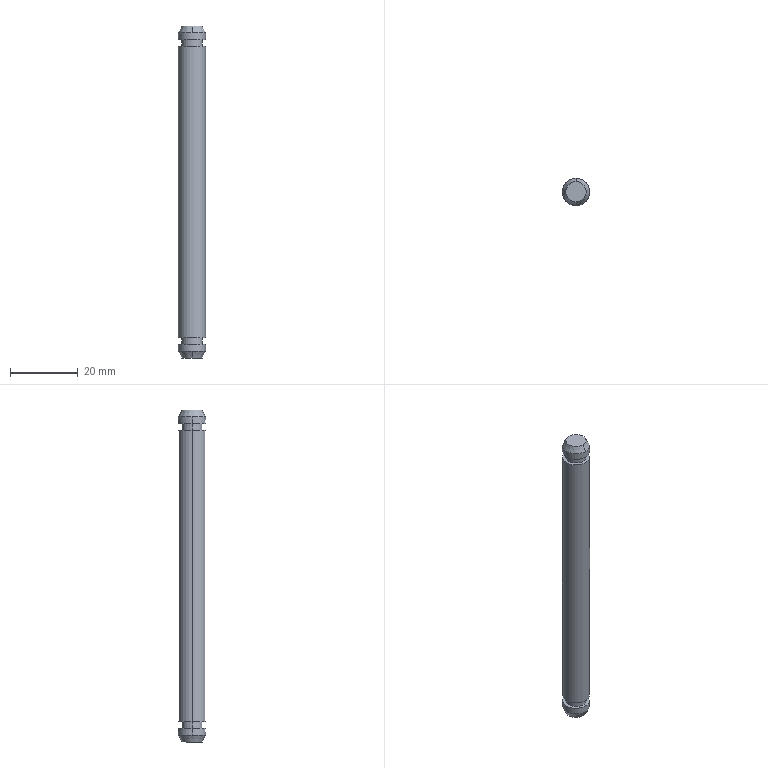Part | SolidWorks | features BaseBody 1 | 1 solid | 20 faces | box 8 x 8 x 98 mm | volume 4792 mm3 | cylinder 10 | plane 6 | cone 4 | commonest cylinder face diameters 8 x6 6 x4
STEP:
#1=CARTESIAN_POINT('',(4.,0.,-43.));
#2=VERTEX_POINT('',#1);
#3=CARTESIAN_POINT('',(-4.,0.,-43.));
#4=VERTEX_POINT('',#3);
#5=CARTESIAN_POINT('',(0.,0.,-43.));
#6=DIRECTION('',(0.,0.,1.));
#7=DIRECTION('',(1.,0.,0.));
#8=AXIS2_PLACEMENT_3D('',#5,#6,#7);
#9=CIRCLE('',#8,4.);
#10=EDGE_CURVE('',#2,#4,#9,.T.);
#11=ORIENTED_EDGE('',*,*,#10,.T.);
#12=CARTESIAN_POINT('',(-4.,0.,43.));
#13=VERTEX_POINT('',#12);
#14=CARTESIAN_POINT('',(-4.,0.,0.));
#15=DIRECTION('',(0.,0.,1.));
#16=VECTOR('',#15,1000.);
#17=LINE('',#14,#16);
#18=EDGE_CURVE('',#4,#13,#17,.T.);
#19=ORIENTED_EDGE('',*,*,#18,.T.);
#20=CARTESIAN_POINT('',(4.,0.,43.));
#21=VERTEX_POINT('',#20);
#22=CARTESIAN_POINT('',(0.,0.,43.));
#23=DIRECTION('',(0.,0.,-1.));
#24=DIRECTION('',(1.,0.,0.));
#25=AXIS2_PLACEMENT_3D('',#22,#23,#24);
#26=CIRCLE('',#25,4.);
#27=EDGE_CURVE('',#13,#21,#26,.T.);
#28=ORIENTED_EDGE('',*,*,#27,.T.);
#29=CARTESIAN_POINT('',(4.,0.,0.));
#30=DIRECTION('',(0.,0.,1.));
#31=VECTOR('',#30,1000.);
#32=LINE('',#29,#31);
#33=EDGE_CURVE('',#2,#21,#32,.T.);
#34=ORIENTED_EDGE('',*,*,#33,.F.);
#35=EDGE_LOOP('',(#11,#19,#28,#34));
#36=FACE_OUTER_BOUND('',#35,.T.);
#37=CARTESIAN_POINT('',(0.,0.,0.));
#38=DIRECTION('',(0.,0.,1.));
#39=DIRECTION('',(1.,0.,0.));
#40=AXIS2_PLACEMENT_3D('',#37,#38,#39);
#41=CYLINDRICAL_SURFACE('',#40,4.);
#42=ADVANCED_FACE('',(#36),#41,.T.);
#43=CARTESIAN_POINT('',(-3.,0.,45.));
#44=VERTEX_POINT('',#43);
#45=CARTESIAN_POINT('',(3.,0.,45.));
#46=VERTEX_POINT('',#45);
#47=CARTESIAN_POINT('',(0.,0.,45.));
#48=DIRECTION('',(0.,0.,-1.));
#49=DIRECTION('',(-1.,0.,0.));
#50=AXIS2_PLACEMENT_3D('',#47,#48,#49);
#51=CIRCLE('',#50,3.);
#52=EDGE_CURVE('',#44,#46,#51,.T.);
#53=ORIENTED_EDGE('',*,*,#52,.T.);
#54=CARTESIAN_POINT('',(3.,0.,43.));
#55=VERTEX_POINT('',#54);
#56=CARTESIAN_POINT('',(3.,0.,0.));
#57=DIRECTION('',(0.,0.,-1.));
#58=VECTOR('',#57,1000.);
#59=LINE('',#56,#58);
#60=EDGE_CURVE('',#46,#55,#59,.T.);
#61=ORIENTED_EDGE('',*,*,#60,.T.);
#62=CARTESIAN_POINT('',(-3.,0.,43.));
#63=VERTEX_POINT('',#62);
#64=CARTESIAN_POINT('',(0.,0.,43.));
#65=DIRECTION('',(0.,0.,1.));
#66=DIRECTION('',(-1.,0.,0.));
#67=AXIS2_PLACEMENT_3D('',#64,#65,#66);
#68=CIRCLE('',#67,3.);
#69=EDGE_CURVE('',#55,#63,#68,.T.);
#70=ORIENTED_EDGE('',*,*,#69,.T.);
#71=CARTESIAN_POINT('',(-3.,0.,0.));
#72=DIRECTION('',(0.,0.,-1.));
#73=VECTOR('',#72,1000.);
#74=LINE('',#71,#73);
#75=EDGE_CURVE('',#44,#63,#74,.T.);
#76=ORIENTED_EDGE('',*,*,#75,.F.);
#77=EDGE_LOOP('',(#53,#61,#70,#76));
#78=FACE_OUTER_BOUND('',#77,.T.);
#79=CARTESIAN_POINT('',(0.,0.,0.));
#80=DIRECTION('',(0.,0.,-1.));
#81=DIRECTION('',(-1.,0.,0.));
#82=AXIS2_PLACEMENT_3D('',#79,#80,#81);
#83=CYLINDRICAL_SURFACE('',#82,3.);
#84=ADVANCED_FACE('',(#78),#83,.T.);
#85=CARTESIAN_POINT('',(3.,0.,-45.));
#86=VERTEX_POINT('',#85);
#87=CARTESIAN_POINT('',(-3.,0.,-45.));
#88=VERTEX_POINT('',#87);
#89=CARTESIAN_POINT('',(0.,0.,-45.));
#90=DIRECTION('',(0.,0.,1.));
#91=DIRECTION('',(1.,0.,0.));
#92=AXIS2_PLACEMENT_3D('',#89,#90,#91);
#93=CIRCLE('',#92,3.);
#94=EDGE_CURVE('',#86,#88,#93,.T.);
#95=ORIENTED_EDGE('',*,*,#94,.T.);
#96=CARTESIAN_POINT('',(-3.,0.,-43.));
#97=VERTEX_POINT('',#96);
#98=CARTESIAN_POINT('',(-3.,0.,0.));
#99=DIRECTION('',(0.,0.,1.));
#100=VECTOR('',#99,1000.);
#101=LINE('',#98,#100);
#102=EDGE_CURVE('',#88,#97,#101,.T.);
#103=ORIENTED_EDGE('',*,*,#102,.T.);
#104=CARTESIAN_POINT('',(3.,0.,-43.));
#105=VERTEX_POINT('',#104);
#106=CARTESIAN_POINT('',(0.,0.,-43.));
#107=DIRECTION('',(0.,0.,-1.));
#108=DIRECTION('',(1.,0.,0.));
#109=AXIS2_PLACEMENT_3D('',#106,#107,#108);
#110=CIRCLE('',#109,3.);
#111=EDGE_CURVE('',#97,#105,#110,.T.);
#112=ORIENTED_EDGE('',*,*,#111,.T.);
#113=CARTESIAN_POINT('',(3.,0.,0.));
#114=DIRECTION('',(0.,0.,1.));
#115=VECTOR('',#114,1000.);
#116=LINE('',#113,#115);
#117=EDGE_CURVE('',#86,#105,#116,.T.);
#118=ORIENTED_EDGE('',*,*,#117,.F.);
#119=EDGE_LOOP('',(#95,#103,#112,#118));
#120=FACE_OUTER_BOUND('',#119,.T.);
#121=CARTESIAN_POINT('',(0.,0.,0.));
#122=DIRECTION('',(0.,0.,1.));
#123=DIRECTION('',(1.,0.,0.));
#124=AXIS2_PLACEMENT_3D('',#121,#122,#123);
#125=CYLINDRICAL_SURFACE('',#124,3.);
#126=ADVANCED_FACE('',(#120),#125,.T.);
#127=CARTESIAN_POINT('',(0.,4.,47.));
#128=VERTEX_POINT('',#127);
#129=CARTESIAN_POINT('',(4.,0.,47.));
#130=VERTEX_POINT('',#129);
#131=CARTESIAN_POINT('',(0.,0.,47.));
#132=DIRECTION('',(0.,0.,-1.));
#133=DIRECTION('',(-1.,0.,0.));
#134=AXIS2_PLACEMENT_3D('',#131,#132,#133);
#135=CIRCLE('',#134,4.);
#136=EDGE_CURVE('',#128,#130,#135,.T.);
#137=ORIENTED_EDGE('',*,*,#136,.T.);
#138=CARTESIAN_POINT('',(4.,0.,45.));
#139=VERTEX_POINT('',#138);
#140=CARTESIAN_POINT('',(4.,0.,0.));
#141=DIRECTION('',(0.,0.,-1.));
#142=VECTOR('',#141,1000.);
#143=LINE('',#140,#142);
#144=EDGE_CURVE('',#130,#139,#143,.T.);
#145=ORIENTED_EDGE('',*,*,#144,.T.);
#146=CARTESIAN_POINT('',(-4.,0.,45.));
#147=VERTEX_POINT('',#146);
#148=CARTESIAN_POINT('',(0.,0.,45.));
#149=DIRECTION('',(0.,0.,1.));
#150=DIRECTION('',(-1.,0.,0.));
#151=AXIS2_PLACEMENT_3D('',#148,#149,#150);
#152=CIRCLE('',#151,4.);
#153=EDGE_CURVE('',#139,#147,#152,.T.);
#154=ORIENTED_EDGE('',*,*,#153,.T.);
#155=CARTESIAN_POINT('',(-4.,0.,47.));
#156=VERTEX_POINT('',#155);
#157=CARTESIAN_POINT('',(-4.,0.,0.));
#158=DIRECTION('',(0.,0.,-1.));
#159=VECTOR('',#158,1000.);
#160=LINE('',#157,#159);
#161=EDGE_CURVE('',#156,#147,#160,.T.);
#162=ORIENTED_EDGE('',*,*,#161,.F.);
#163=CARTESIAN_POINT('',(0.,0.,47.));
#164=DIRECTION('',(0.,0.,-1.));
#165=DIRECTION('',(-1.,0.,0.));
#166=AXIS2_PLACEMENT_3D('',#163,#164,#165);
#167=CIRCLE('',#166,4.);
#168=EDGE_CURVE('',#156,#128,#167,.T.);
#169=ORIENTED_EDGE('',*,*,#168,.T.);
#170=EDGE_LOOP('',(#137,#145,#154,#162,#169));
#171=FACE_OUTER_BOUND('',#170,.T.);
#172=CARTESIAN_POINT('',(0.,0.,0.));
#173=DIRECTION('',(0.,0.,-1.));
#174=DIRECTION('',(-1.,0.,0.));
#175=AXIS2_PLACEMENT_3D('',#172,#173,#174);
#176=CYLINDRICAL_SURFACE('',#175,4.);
#177=ADVANCED_FACE('',(#171),#176,.T.);
#178=CARTESIAN_POINT('',(0.,4.,-47.));
#179=VERTEX_POINT('',#178);
#180=CARTESIAN_POINT('',(-4.,0.,-47.));
#181=VERTEX_POINT('',#180);
#182=CARTESIAN_POINT('',(0.,0.,-47.));
#183=DIRECTION('',(0.,0.,1.));
#184=DIRECTION('',(1.,0.,0.));
#185=AXIS2_PLACEMENT_3D('',#182,#183,#184);
#186=CIRCLE('',#185,4.);
#187=EDGE_CURVE('',#179,#181,#186,.T.);
#188=ORIENTED_EDGE('',*,*,#187,.T.);
#189=CARTESIAN_POINT('',(-4.,0.,-45.));
#190=VERTEX_POINT('',#189);
#191=CARTESIAN_POINT('',(-4.,0.,0.));
#192=DIRECTION('',(0.,0.,1.));
#193=VECTOR('',#192,1000.);
#194=LINE('',#191,#193);
#195=EDGE_CURVE('',#181,#190,#194,.T.);
#196=ORIENTED_EDGE('',*,*,#195,.T.);
#197=CARTESIAN_POINT('',(4.,0.,-45.));
#198=VERTEX_POINT('',#197);
#199=CARTESIAN_POINT('',(0.,0.,-45.));
#200=DIRECTION('',(0.,0.,-1.));
#201=DIRECTION('',(1.,0.,0.));
#202=AXIS2_PLACEMENT_3D('',#199,#200,#201);
#203=CIRCLE('',#202,4.);
#204=EDGE_CURVE('',#190,#198,#203,.T.);
#205=ORIENTED_EDGE('',*,*,#204,.T.);
#206=CARTESIAN_POINT('',(4.,0.,-47.));
#207=VERTEX_POINT('',#206);
#208=CARTESIAN_POINT('',(4.,0.,0.));
#209=DIRECTION('',(0.,0.,1.));
#210=VECTOR('',#209,1000.);
#211=LINE('',#208,#210);
#212=EDGE_CURVE('',#207,#198,#211,.T.);
#213=ORIENTED_EDGE('',*,*,#212,.F.);
#214=CARTESIAN_POINT('',(0.,0.,-47.));
#215=DIRECTION('',(0.,0.,1.));
#216=DIRECTION('',(1.,0.,0.));
#217=AXIS2_PLACEMENT_3D('',#214,#215,#216);
#218=CIRCLE('',#217,4.);
#219=EDGE_CURVE('',#207,#179,#218,.T.);
#220=ORIENTED_EDGE('',*,*,#219,.T.);
#221=EDGE_LOOP('',(#188,#196,#205,#213,#220));
#222=FACE_OUTER_BOUND('',#221,.T.);
#223=CARTESIAN_POINT('',(0.,0.,0.));
#224=DIRECTION('',(0.,0.,1.));
#225=DIRECTION('',(1.,0.,0.));
#226=AXIS2_PLACEMENT_3D('',#223,#224,#225);
#227=CYLINDRICAL_SURFACE('',#226,4.);
#228=ADVANCED_FACE('',(#222),#227,.T.);
#229=CARTESIAN_POINT('',(0.,3.,49.));
#230=VERTEX_POINT('',#229);
#231=CARTESIAN_POINT('',(0.,-3.,49.));
#232=VERTEX_POINT('',#231);
#233=CARTESIAN_POINT('',(0.,0.,49.));
#234=DIRECTION('',(0.,0.,-1.));
#235=DIRECTION('',(0.,1.,0.));
#236=AXIS2_PLACEMENT_3D('',#233,#234,#235);
#237=CIRCLE('',#236,3.);
#238=EDGE_CURVE('',#230,#232,#237,.T.);
#239=ORIENTED_EDGE('',*,*,#238,.T.);
#240=CARTESIAN_POINT('',(0.,-4.,47.));
#241=VERTEX_POINT('',#240);
#242=CARTESIAN_POINT('',(0.,-4.,47.));
#243=DIRECTION('',(0.,-0.4472,-0.8944));
#244=VECTOR('',#243,1000.);
#245=LINE('',#242,#244);
#246=EDGE_CURVE('',#232,#241,#245,.T.);
#247=ORIENTED_EDGE('',*,*,#246,.T.);
#248=CARTESIAN_POINT('',(0.,0.,47.));
#249=DIRECTION('',(0.,0.,-1.));
#250=DIRECTION('',(-1.,0.,0.));
#251=AXIS2_PLACEMENT_3D('',#248,#249,#250);
#252=CIRCLE('',#251,4.);
#253=EDGE_CURVE('',#130,#241,#252,.T.);
#254=ORIENTED_EDGE('',*,*,#253,.F.);
#255=ORIENTED_EDGE('',*,*,#136,.F.);
#256=CARTESIAN_POINT('',(0.,4.,47.));
#257=DIRECTION('',(0.,0.4472,-0.8944));
#258=VECTOR('',#257,1000.);
#259=LINE('',#256,#258);
#260=EDGE_CURVE('',#230,#128,#259,.T.);
#261=ORIENTED_EDGE('',*,*,#260,.F.);
#262=EDGE_LOOP('',(#239,#247,#254,#255,#261));
#263=FACE_OUTER_BOUND('',#262,.T.);
#264=CARTESIAN_POINT('',(0.,0.,47.));
#265=DIRECTION('',(0.,0.,-1.));
#266=DIRECTION('',(0.,1.,0.));
#267=AXIS2_PLACEMENT_3D('',#264,#265,#266);
#268=CONICAL_SURFACE('',#267,4.,0.4636);
#269=ADVANCED_FACE('',(#263),#268,.T.);
#270=CARTESIAN_POINT('',(0.,-3.,-49.));
#271=VERTEX_POINT('',#270);
#272=CARTESIAN_POINT('',(0.,3.,-49.));
#273=VERTEX_POINT('',#272);
#274=CARTESIAN_POINT('',(0.,0.,-49.));
#275=DIRECTION('',(0.,0.,1.));
#276=DIRECTION('',(0.,-1.,0.));
#277=AXIS2_PLACEMENT_3D('',#274,#275,#276);
#278=CIRCLE('',#277,3.);
#279=EDGE_CURVE('',#271,#273,#278,.T.);
#280=ORIENTED_EDGE('',*,*,#279,.T.);
#281=CARTESIAN_POINT('',(0.,4.,-47.));
#282=DIRECTION('',(0.,0.4472,0.8944));
#283=VECTOR('',#282,1000.);
#284=LINE('',#281,#283);
#285=EDGE_CURVE('',#273,#179,#284,.T.);
#286=ORIENTED_EDGE('',*,*,#285,.T.);
#287=ORIENTED_EDGE('',*,*,#219,.F.);
#288=CARTESIAN_POINT('',(0.,-4.,-47.));
#289=VERTEX_POINT('',#288);
#290=CARTESIAN_POINT('',(0.,0.,-47.));
#291=DIRECTION('',(0.,0.,1.));
#292=DIRECTION('',(1.,0.,0.));
#293=AXIS2_PLACEMENT_3D('',#290,#291,#292);
#294=CIRCLE('',#293,4.);
#295=EDGE_CURVE('',#289,#207,#294,.T.);
#296=ORIENTED_EDGE('',*,*,#295,.F.);
#297=CARTESIAN_POINT('',(0.,-4.,-47.));
#298=DIRECTION('',(0.,-0.4472,0.8944));
#299=VECTOR('',#298,1000.);
#300=LINE('',#297,#299);
#301=EDGE_CURVE('',#271,#289,#300,.T.);
#302=ORIENTED_EDGE('',*,*,#301,.F.);
#303=EDGE_LOOP('',(#280,#286,#287,#296,#302));
#304=FACE_OUTER_BOUND('',#303,.T.);
#305=CARTESIAN_POINT('',(0.,0.,-47.));
#306=DIRECTION('',(0.,0.,1.));
#307=DIRECTION('',(0.,-1.,0.));
#308=AXIS2_PLACEMENT_3D('',#305,#306,#307);
#309=CONICAL_SURFACE('',#308,4.,0.4636);
#310=ADVANCED_FACE('',(#304),#309,.T.);
#311=ORIENTED_EDGE('',*,*,#18,.F.);
#312=CARTESIAN_POINT('',(0.,0.,-43.));
#313=DIRECTION('',(0.,0.,1.));
#314=DIRECTION('',(1.,0.,0.));
#315=AXIS2_PLACEMENT_3D('',#312,#313,#314);
#316=CIRCLE('',#315,4.);
#317=EDGE_CURVE('',#4,#2,#316,.T.);
#318=ORIENTED_EDGE('',*,*,#317,.T.);
#319=ORIENTED_EDGE('',*,*,#33,.T.);
#320=CARTESIAN_POINT('',(0.,0.,43.));
#321=DIRECTION('',(0.,0.,-1.));
#322=DIRECTION('',(1.,0.,0.));
#323=AXIS2_PLACEMENT_3D('',#320,#321,#322);
#324=CIRCLE('',#323,4.);
#325=EDGE_CURVE('',#21,#13,#324,.T.);
#326=ORIENTED_EDGE('',*,*,#325,.T.);
#327=EDGE_LOOP('',(#311,#318,#319,#326));
#328=FACE_OUTER_BOUND('',#327,.T.);
#329=CARTESIAN_POINT('',(0.,0.,0.));
#330=DIRECTION('',(0.,0.,1.));
#331=DIRECTION('',(1.,0.,0.));
#332=AXIS2_PLACEMENT_3D('',#329,#330,#331);
#333=CYLINDRICAL_SURFACE('',#332,4.);
#334=ADVANCED_FACE('',(#328),#333,.T.);
#335=ORIENTED_EDGE('',*,*,#325,.F.);
#336=ORIENTED_EDGE('',*,*,#27,.F.);
#337=EDGE_LOOP('',(#335,#336));
#338=FACE_OUTER_BOUND('',#337,.T.);
#339=CARTESIAN_POINT('',(0.,0.,43.));
#340=DIRECTION('',(0.,0.,1.));
#341=DIRECTION('',(-1.,0.,0.));
#342=AXIS2_PLACEMENT_3D('',#339,#340,#341);
#343=CIRCLE('',#342,3.);
#344=EDGE_CURVE('',#63,#55,#343,.T.);
#345=ORIENTED_EDGE('',*,*,#344,.F.);
#346=ORIENTED_EDGE('',*,*,#69,.F.);
#347=EDGE_LOOP('',(#345,#346));
#348=FACE_BOUND('',#347,.T.);
#349=CARTESIAN_POINT('',(0.,4.,43.));
#350=DIRECTION('',(0.,0.,-1.));
#351=DIRECTION('',(-1.,0.,0.));
#352=AXIS2_PLACEMENT_3D('',#349,#350,#351);
#353=PLANE('',#352);
#354=ADVANCED_FACE('',(#338,#348),#353,.F.);
#355=ORIENTED_EDGE('',*,*,#10,.F.);
#356=ORIENTED_EDGE('',*,*,#317,.F.);
#357=EDGE_LOOP('',(#355,#356));
#358=FACE_OUTER_BOUND('',#357,.T.);
#359=CARTESIAN_POINT('',(0.,0.,-43.));
#360=DIRECTION('',(0.,0.,-1.));
#361=DIRECTION('',(1.,0.,0.));
#362=AXIS2_PLACEMENT_3D('',#359,#360,#361);
#363=CIRCLE('',#362,3.);
#364=EDGE_CURVE('',#105,#97,#363,.T.);
#365=ORIENTED_EDGE('',*,*,#364,.F.);
#366=ORIENTED_EDGE('',*,*,#111,.F.);
#367=EDGE_LOOP('',(#365,#366));
#368=FACE_BOUND('',#367,.T.);
#369=CARTESIAN_POINT('',(0.,4.,-43.));
#370=DIRECTION('',(0.,0.,1.));
#371=DIRECTION('',(1.,0.,0.));
#372=AXIS2_PLACEMENT_3D('',#369,#370,#371);
#373=PLANE('',#372);
#374=ADVANCED_FACE('',(#358,#368),#373,.F.);
#375=ORIENTED_EDGE('',*,*,#60,.F.);
#376=CARTESIAN_POINT('',(0.,0.,45.));
#377=DIRECTION('',(0.,0.,-1.));
#378=DIRECTION('',(-1.,0.,0.));
#379=AXIS2_PLACEMENT_3D('',#376,#377,#378);
#380=CIRCLE('',#379,3.);
#381=EDGE_CURVE('',#46,#44,#380,.T.);
#382=ORIENTED_EDGE('',*,*,#381,.T.);
#383=ORIENTED_EDGE('',*,*,#75,.T.);
#384=ORIENTED_EDGE('',*,*,#344,.T.);
#385=EDGE_LOOP('',(#375,#382,#383,#384));
#386=FACE_OUTER_BOUND('',#385,.T.);
#387=CARTESIAN_POINT('',(0.,0.,0.));
#388=DIRECTION('',(0.,0.,-1.));
#389=DIRECTION('',(-1.,0.,0.));
#390=AXIS2_PLACEMENT_3D('',#387,#388,#389);
#391=CYLINDRICAL_SURFACE('',#390,3.);
#392=ADVANCED_FACE('',(#386),#391,.T.);
#393=ORIENTED_EDGE('',*,*,#102,.F.);
#394=CARTESIAN_POINT('',(0.,0.,-45.));
#395=DIRECTION('',(0.,0.,1.));
#396=DIRECTION('',(1.,0.,0.));
#397=AXIS2_PLACEMENT_3D('',#394,#395,#396);
#398=CIRCLE('',#397,3.);
#399=EDGE_CURVE('',#88,#86,#398,.T.);
#400=ORIENTED_EDGE('',*,*,#399,.T.);
#401=ORIENTED_EDGE('',*,*,#117,.T.);
#402=ORIENTED_EDGE('',*,*,#364,.T.);
#403=EDGE_LOOP('',(#393,#400,#401,#402));
#404=FACE_OUTER_BOUND('',#403,.T.);
#405=CARTESIAN_POINT('',(0.,0.,0.));
#406=DIRECTION('',(0.,0.,1.));
#407=DIRECTION('',(1.,0.,0.));
#408=AXIS2_PLACEMENT_3D('',#405,#406,#407);
#409=CYLINDRICAL_SURFACE('',#408,3.);
#410=ADVANCED_FACE('',(#404),#409,.T.);
#411=ORIENTED_EDGE('',*,*,#52,.F.);
#412=ORIENTED_EDGE('',*,*,#381,.F.);
#413=EDGE_LOOP('',(#411,#412));
#414=FACE_BOUND('',#413,.T.);
#415=CARTESIAN_POINT('',(0.,0.,45.));
#416=DIRECTION('',(0.,0.,1.));
#417=DIRECTION('',(-1.,0.,0.));
#418=AXIS2_PLACEMENT_3D('',#415,#416,#417);
#419=CIRCLE('',#418,4.);
#420=EDGE_CURVE('',#147,#139,#419,.T.);
#421=ORIENTED_EDGE('',*,*,#420,.F.);
#422=ORIENTED_EDGE('',*,*,#153,.F.);
#423=EDGE_LOOP('',(#421,#422));
#424=FACE_OUTER_BOUND('',#423,.T.);
#425=CARTESIAN_POINT('',(0.,3.,45.));
#426=DIRECTION('',(0.,0.,1.));
#427=DIRECTION('',(1.,0.,0.));
#428=AXIS2_PLACEMENT_3D('',#425,#426,#427);
#429=PLANE('',#428);
#430=ADVANCED_FACE('',(#414,#424),#429,.F.);
#431=ORIENTED_EDGE('',*,*,#94,.F.);
#432=ORIENTED_EDGE('',*,*,#399,.F.);
#433=EDGE_LOOP('',(#431,#432));
#434=FACE_BOUND('',#433,.T.);
#435=CARTESIAN_POINT('',(0.,0.,-45.));
#436=DIRECTION('',(0.,0.,-1.));
#437=DIRECTION('',(1.,0.,0.));
#438=AXIS2_PLACEMENT_3D('',#435,#436,#437);
#439=CIRCLE('',#438,4.);
#440=EDGE_CURVE('',#198,#190,#439,.T.);
#441=ORIENTED_EDGE('',*,*,#440,.F.);
#442=ORIENTED_EDGE('',*,*,#204,.F.);
#443=EDGE_LOOP('',(#441,#442));
#444=FACE_OUTER_BOUND('',#443,.T.);
#445=CARTESIAN_POINT('',(0.,3.,-45.));
#446=DIRECTION('',(0.,0.,-1.));
#447=DIRECTION('',(-1.,0.,0.));
#448=AXIS2_PLACEMENT_3D('',#445,#446,#447);
#449=PLANE('',#448);
#450=ADVANCED_FACE('',(#434,#444),#449,.F.);
#451=ORIENTED_EDGE('',*,*,#144,.F.);
#452=ORIENTED_EDGE('',*,*,#253,.T.);
#453=CARTESIAN_POINT('',(0.,0.,47.));
#454=DIRECTION('',(0.,0.,-1.));
#455=DIRECTION('',(-1.,0.,0.));
#456=AXIS2_PLACEMENT_3D('',#453,#454,#455);
#457=CIRCLE('',#456,4.);
#458=EDGE_CURVE('',#241,#156,#457,.T.);
#459=ORIENTED_EDGE('',*,*,#458,.T.);
#460=ORIENTED_EDGE('',*,*,#161,.T.);
#461=ORIENTED_EDGE('',*,*,#420,.T.);
#462=EDGE_LOOP('',(#451,#452,#459,#460,#461));
#463=FACE_OUTER_BOUND('',#462,.T.);
#464=CARTESIAN_POINT('',(0.,0.,0.));
#465=DIRECTION('',(0.,0.,-1.));
#466=DIRECTION('',(-1.,0.,0.));
#467=AXIS2_PLACEMENT_3D('',#464,#465,#466);
#468=CYLINDRICAL_SURFACE('',#467,4.);
#469=ADVANCED_FACE('',(#463),#468,.T.);
#470=ORIENTED_EDGE('',*,*,#195,.F.);
#471=CARTESIAN_POINT('',(0.,0.,-47.));
#472=DIRECTION('',(0.,0.,1.));
#473=DIRECTION('',(1.,0.,0.));
#474=AXIS2_PLACEMENT_3D('',#471,#472,#473);
#475=CIRCLE('',#474,4.);
#476=EDGE_CURVE('',#181,#289,#475,.T.);
#477=ORIENTED_EDGE('',*,*,#476,.T.);
#478=ORIENTED_EDGE('',*,*,#295,.T.);
#479=ORIENTED_EDGE('',*,*,#212,.T.);
#480=ORIENTED_EDGE('',*,*,#440,.T.);
#481=EDGE_LOOP('',(#470,#477,#478,#479,#480));
#482=FACE_OUTER_BOUND('',#481,.T.);
#483=CARTESIAN_POINT('',(0.,0.,0.));
#484=DIRECTION('',(0.,0.,1.));
#485=DIRECTION('',(1.,0.,0.));
#486=AXIS2_PLACEMENT_3D('',#483,#484,#485);
#487=CYLINDRICAL_SURFACE('',#486,4.);
#488=ADVANCED_FACE('',(#482),#487,.T.);
#489=ORIENTED_EDGE('',*,*,#246,.F.);
#490=CARTESIAN_POINT('',(0.,0.,49.));
#491=DIRECTION('',(0.,0.,-1.));
#492=DIRECTION('',(0.,1.,0.));
#493=AXIS2_PLACEMENT_3D('',#490,#491,#492);
#494=CIRCLE('',#493,3.);
#495=EDGE_CURVE('',#232,#230,#494,.T.);
#496=ORIENTED_EDGE('',*,*,#495,.T.);
#497=ORIENTED_EDGE('',*,*,#260,.T.);
#498=ORIENTED_EDGE('',*,*,#168,.F.);
#499=ORIENTED_EDGE('',*,*,#458,.F.);
#500=EDGE_LOOP('',(#489,#496,#497,#498,#499));
#501=FACE_OUTER_BOUND('',#500,.T.);
#502=CARTESIAN_POINT('',(0.,0.,47.));
#503=DIRECTION('',(0.,0.,-1.));
#504=DIRECTION('',(0.,1.,0.));
#505=AXIS2_PLACEMENT_3D('',#502,#503,#504);
#506=CONICAL_SURFACE('',#505,4.,0.4636);
#507=ADVANCED_FACE('',(#501),#506,.T.);
#508=ORIENTED_EDGE('',*,*,#285,.F.);
#509=CARTESIAN_POINT('',(0.,0.,-49.));
#510=DIRECTION('',(0.,0.,1.));
#511=DIRECTION('',(0.,-1.,0.));
#512=AXIS2_PLACEMENT_3D('',#509,#510,#511);
#513=CIRCLE('',#512,3.);
#514=EDGE_CURVE('',#273,#271,#513,.T.);
#515=ORIENTED_EDGE('',*,*,#514,.T.);
#516=ORIENTED_EDGE('',*,*,#301,.T.);
#517=ORIENTED_EDGE('',*,*,#476,.F.);
#518=ORIENTED_EDGE('',*,*,#187,.F.);
#519=EDGE_LOOP('',(#508,#515,#516,#517,#518));
#520=FACE_OUTER_BOUND('',#519,.T.);
#521=CARTESIAN_POINT('',(0.,0.,-47.));
#522=DIRECTION('',(0.,0.,1.));
#523=DIRECTION('',(0.,-1.,0.));
#524=AXIS2_PLACEMENT_3D('',#521,#522,#523);
#525=CONICAL_SURFACE('',#524,4.,0.4636);
#526=ADVANCED_FACE('',(#520),#525,.T.);
#527=ORIENTED_EDGE('',*,*,#238,.F.);
#528=ORIENTED_EDGE('',*,*,#495,.F.);
#529=EDGE_LOOP('',(#527,#528));
#530=FACE_OUTER_BOUND('',#529,.T.);
#531=CARTESIAN_POINT('',(0.,3.,49.));
#532=DIRECTION('',(0.,0.,-1.));
#533=DIRECTION('',(-1.,0.,0.));
#534=AXIS2_PLACEMENT_3D('',#531,#532,#533);
#535=PLANE('',#534);
#536=ADVANCED_FACE('',(#530),#535,.F.);
#537=ORIENTED_EDGE('',*,*,#279,.F.);
#538=ORIENTED_EDGE('',*,*,#514,.F.);
#539=EDGE_LOOP('',(#537,#538));
#540=FACE_OUTER_BOUND('',#539,.T.);
#541=CARTESIAN_POINT('',(0.,3.,-49.));
#542=DIRECTION('',(0.,0.,1.));
#543=DIRECTION('',(1.,0.,0.));
#544=AXIS2_PLACEMENT_3D('',#541,#542,#543);
#545=PLANE('',#544);
#546=ADVANCED_FACE('',(#540),#545,.F.);
#547=CLOSED_SHELL('',(#42,#84,#126,#177,#228,#269,#310,#334,#354,#374,#392,#410,#430,#450,#469,#488,#507,#526,#536,#546));
#548=MANIFOLD_SOLID_BREP('',#547);
#549=CARTESIAN_POINT('',(0.,0.,0.));
#550=DIRECTION('',(0.,0.,1.));
#551=DIRECTION('',(1.,0.,0.));
#552=AXIS2_PLACEMENT_3D('',#549,#550,#551);
#553=(LENGTH_UNIT()NAMED_UNIT(*)SI_UNIT(.MILLI.,.METRE.));
#554=UNCERTAINTY_MEASURE_WITH_UNIT(LENGTH_MEASURE(0.00001),#553,'','');
#555=(NAMED_UNIT(*)PLANE_ANGLE_UNIT()SI_UNIT($,.RADIAN.));
#556=(NAMED_UNIT(*)SI_UNIT($,.STERADIAN.)SOLID_ANGLE_UNIT());
#557=(GEOMETRIC_REPRESENTATION_CONTEXT(3)GLOBAL_UNCERTAINTY_ASSIGNED_CONTEXT((#554))GLOBAL_UNIT_ASSIGNED_CONTEXT((#553,#555,#556))REPRESENTATION_CONTEXT('',''));
#558=ADVANCED_BREP_SHAPE_REPRESENTATION('',(#548,#552),#557);